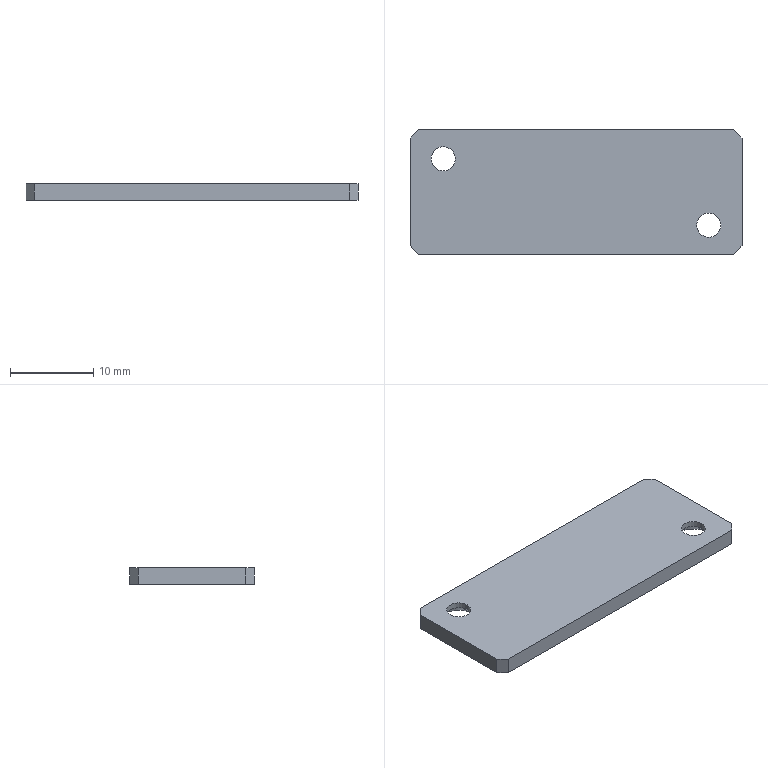Part | NX | features BREP 1 | 1 solid | 18 faces | box 40 x 15 x 2 mm | volume 1150 mm3 | plane 10 | cone 4 | cylinder 4 | commonest cylinder face diameters 2.9 x4
STEP:
#1=CARTESIAN_POINT('',(20.,6.5,1.));
#2=VERTEX_POINT('',#1);
#3=CARTESIAN_POINT('',(19.,7.5,1.));
#4=VERTEX_POINT('',#3);
#5=CARTESIAN_POINT('',(13.25,13.25,1.));
#6=DIRECTION('',(-0.7071,0.7071,0.));
#7=VECTOR('',#6,1000.);
#8=LINE('',#5,#7);
#9=EDGE_CURVE('',#2,#4,#8,.T.);
#10=ORIENTED_EDGE('',*,*,#9,.F.);
#11=CARTESIAN_POINT('',(20.,6.5,-1.));
#12=VERTEX_POINT('',#11);
#13=CARTESIAN_POINT('',(20.,6.5,1.));
#14=DIRECTION('',(0.,0.,1.));
#15=VECTOR('',#14,1000.);
#16=LINE('',#13,#15);
#17=EDGE_CURVE('',#12,#2,#16,.T.);
#18=ORIENTED_EDGE('',*,*,#17,.F.);
#19=CARTESIAN_POINT('',(19.,7.5,-1.));
#20=VERTEX_POINT('',#19);
#21=CARTESIAN_POINT('',(19.,7.5,-1.));
#22=DIRECTION('',(0.7071,-0.7071,0.));
#23=VECTOR('',#22,1000.);
#24=LINE('',#21,#23);
#25=EDGE_CURVE('',#20,#12,#24,.T.);
#26=ORIENTED_EDGE('',*,*,#25,.F.);
#27=CARTESIAN_POINT('',(19.,7.5,-1.));
#28=DIRECTION('',(0.,0.,-1.));
#29=VECTOR('',#28,1000.);
#30=LINE('',#27,#29);
#31=EDGE_CURVE('',#4,#20,#30,.T.);
#32=ORIENTED_EDGE('',*,*,#31,.F.);
#33=EDGE_LOOP('',(#10,#18,#26,#32));
#34=FACE_BOUND('',#33,.T.);
#35=CARTESIAN_POINT('',(19.,7.5,1.));
#36=DIRECTION('',(0.7071,0.7071,0.));
#37=DIRECTION('',(0.,0.,1.));
#38=AXIS2_PLACEMENT_3D('',#35,#36,#37);
#39=PLANE('',#38);
#40=ADVANCED_FACE('',(#34),#39,.T.);
#41=CARTESIAN_POINT('',(19.,-7.5,1.));
#42=VERTEX_POINT('',#41);
#43=CARTESIAN_POINT('',(20.,-6.5,1.));
#44=VERTEX_POINT('',#43);
#45=CARTESIAN_POINT('',(13.25,-13.25,1.));
#46=DIRECTION('',(0.7071,0.7071,0.));
#47=VECTOR('',#46,1000.);
#48=LINE('',#45,#47);
#49=EDGE_CURVE('',#42,#44,#48,.T.);
#50=ORIENTED_EDGE('',*,*,#49,.F.);
#51=CARTESIAN_POINT('',(19.,-7.5,-1.));
#52=VERTEX_POINT('',#51);
#53=CARTESIAN_POINT('',(19.,-7.5,1.));
#54=DIRECTION('',(0.,0.,1.));
#55=VECTOR('',#54,1000.);
#56=LINE('',#53,#55);
#57=EDGE_CURVE('',#52,#42,#56,.T.);
#58=ORIENTED_EDGE('',*,*,#57,.F.);
#59=CARTESIAN_POINT('',(20.,-6.5,-1.));
#60=VERTEX_POINT('',#59);
#61=CARTESIAN_POINT('',(20.,-6.5,-1.));
#62=DIRECTION('',(-0.7071,-0.7071,0.));
#63=VECTOR('',#62,1000.);
#64=LINE('',#61,#63);
#65=EDGE_CURVE('',#60,#52,#64,.T.);
#66=ORIENTED_EDGE('',*,*,#65,.F.);
#67=CARTESIAN_POINT('',(20.,-6.5,1.));
#68=DIRECTION('',(0.,0.,-1.));
#69=VECTOR('',#68,1000.);
#70=LINE('',#67,#69);
#71=EDGE_CURVE('',#44,#60,#70,.T.);
#72=ORIENTED_EDGE('',*,*,#71,.F.);
#73=EDGE_LOOP('',(#50,#58,#66,#72));
#74=FACE_BOUND('',#73,.T.);
#75=CARTESIAN_POINT('',(20.,-6.5,1.));
#76=DIRECTION('',(-0.7071,0.7071,0.));
#77=DIRECTION('',(0.,0.,-1.));
#78=AXIS2_PLACEMENT_3D('',#75,#76,#77);
#79=PLANE('',#78);
#80=ADVANCED_FACE('',(#74),#79,.F.);
#81=CARTESIAN_POINT('',(-19.,7.5,1.));
#82=VERTEX_POINT('',#81);
#83=CARTESIAN_POINT('',(-20.,6.5,1.));
#84=VERTEX_POINT('',#83);
#85=CARTESIAN_POINT('',(-13.25,13.25,1.));
#86=DIRECTION('',(-0.7071,-0.7071,0.));
#87=VECTOR('',#86,1000.);
#88=LINE('',#85,#87);
#89=EDGE_CURVE('',#82,#84,#88,.T.);
#90=ORIENTED_EDGE('',*,*,#89,.F.);
#91=CARTESIAN_POINT('',(-19.,7.5,-1.));
#92=VERTEX_POINT('',#91);
#93=CARTESIAN_POINT('',(-19.,7.5,1.));
#94=DIRECTION('',(0.,0.,1.));
#95=VECTOR('',#94,1000.);
#96=LINE('',#93,#95);
#97=EDGE_CURVE('',#92,#82,#96,.T.);
#98=ORIENTED_EDGE('',*,*,#97,.F.);
#99=CARTESIAN_POINT('',(-20.,6.5,-1.));
#100=VERTEX_POINT('',#99);
#101=CARTESIAN_POINT('',(-20.,6.5,-1.));
#102=DIRECTION('',(0.7071,0.7071,0.));
#103=VECTOR('',#102,1000.);
#104=LINE('',#101,#103);
#105=EDGE_CURVE('',#100,#92,#104,.T.);
#106=ORIENTED_EDGE('',*,*,#105,.F.);
#107=CARTESIAN_POINT('',(-20.,6.5,1.));
#108=DIRECTION('',(0.,0.,-1.));
#109=VECTOR('',#108,1000.);
#110=LINE('',#107,#109);
#111=EDGE_CURVE('',#84,#100,#110,.T.);
#112=ORIENTED_EDGE('',*,*,#111,.F.);
#113=EDGE_LOOP('',(#90,#98,#106,#112));
#114=FACE_BOUND('',#113,.T.);
#115=CARTESIAN_POINT('',(-20.,6.5,1.));
#116=DIRECTION('',(0.7071,-0.7071,0.));
#117=DIRECTION('',(0.,0.,-1.));
#118=AXIS2_PLACEMENT_3D('',#115,#116,#117);
#119=PLANE('',#118);
#120=ADVANCED_FACE('',(#114),#119,.F.);
#121=CARTESIAN_POINT('',(-20.,-6.5,1.));
#122=VERTEX_POINT('',#121);
#123=CARTESIAN_POINT('',(-19.,-7.5,1.));
#124=VERTEX_POINT('',#123);
#125=CARTESIAN_POINT('',(-13.25,-13.25,1.));
#126=DIRECTION('',(0.7071,-0.7071,0.));
#127=VECTOR('',#126,1000.);
#128=LINE('',#125,#127);
#129=EDGE_CURVE('',#122,#124,#128,.T.);
#130=ORIENTED_EDGE('',*,*,#129,.F.);
#131=CARTESIAN_POINT('',(-20.,-6.5,-1.));
#132=VERTEX_POINT('',#131);
#133=CARTESIAN_POINT('',(-20.,-6.5,1.));
#134=DIRECTION('',(0.,0.,1.));
#135=VECTOR('',#134,1000.);
#136=LINE('',#133,#135);
#137=EDGE_CURVE('',#132,#122,#136,.T.);
#138=ORIENTED_EDGE('',*,*,#137,.F.);
#139=CARTESIAN_POINT('',(-19.,-7.5,-1.));
#140=VERTEX_POINT('',#139);
#141=CARTESIAN_POINT('',(-19.,-7.5,-1.));
#142=DIRECTION('',(-0.7071,0.7071,0.));
#143=VECTOR('',#142,1000.);
#144=LINE('',#141,#143);
#145=EDGE_CURVE('',#140,#132,#144,.T.);
#146=ORIENTED_EDGE('',*,*,#145,.F.);
#147=CARTESIAN_POINT('',(-19.,-7.5,-1.));
#148=DIRECTION('',(0.,0.,-1.));
#149=VECTOR('',#148,1000.);
#150=LINE('',#147,#149);
#151=EDGE_CURVE('',#124,#140,#150,.T.);
#152=ORIENTED_EDGE('',*,*,#151,.F.);
#153=EDGE_LOOP('',(#130,#138,#146,#152));
#154=FACE_BOUND('',#153,.T.);
#155=CARTESIAN_POINT('',(-19.,-7.5,1.));
#156=DIRECTION('',(-0.7071,-0.7071,0.));
#157=DIRECTION('',(0.,0.,1.));
#158=AXIS2_PLACEMENT_3D('',#155,#156,#157);
#159=PLANE('',#158);
#160=ADVANCED_FACE('',(#154),#159,.T.);
#161=CARTESIAN_POINT('',(-14.55,4.,0.3));
#162=VERTEX_POINT('',#161);
#163=CARTESIAN_POINT('',(-13.25,4.,-1.));
#164=VERTEX_POINT('',#163);
#165=CARTESIAN_POINT('',(-13.25,4.,-1.));
#166=DIRECTION('',(0.7071,0.,-0.7071));
#167=VECTOR('',#166,1000.);
#168=LINE('',#165,#167);
#169=EDGE_CURVE('',#162,#164,#168,.T.);
#170=ORIENTED_EDGE('',*,*,#169,.F.);
#171=CARTESIAN_POINT('',(-17.45,4.,0.3));
#172=VERTEX_POINT('',#171);
#173=CARTESIAN_POINT('',(-16.,4.,0.3));
#174=DIRECTION('',(0.,0.,-1.));
#175=DIRECTION('',(-1.,0.,0.));
#176=AXIS2_PLACEMENT_3D('',#173,#174,#175);
#177=CIRCLE('',#176,1.45);
#178=EDGE_CURVE('',#172,#162,#177,.T.);
#179=ORIENTED_EDGE('',*,*,#178,.F.);
#180=CARTESIAN_POINT('',(-18.75,4.,-1.));
#181=VERTEX_POINT('',#180);
#182=CARTESIAN_POINT('',(-18.75,4.,-1.));
#183=DIRECTION('',(-0.7071,0.,-0.7071));
#184=VECTOR('',#183,1000.);
#185=LINE('',#182,#184);
#186=EDGE_CURVE('',#172,#181,#185,.T.);
#187=ORIENTED_EDGE('',*,*,#186,.T.);
#188=CARTESIAN_POINT('',(-16.,4.,-1.));
#189=DIRECTION('',(0.,0.,-1.));
#190=DIRECTION('',(-1.,0.,0.));
#191=AXIS2_PLACEMENT_3D('',#188,#189,#190);
#192=CIRCLE('',#191,2.75);
#193=EDGE_CURVE('',#181,#164,#192,.T.);
#194=ORIENTED_EDGE('',*,*,#193,.T.);
#195=EDGE_LOOP('',(#170,#179,#187,#194));
#196=FACE_BOUND('',#195,.T.);
#197=CARTESIAN_POINT('',(-16.,4.,-1.));
#198=DIRECTION('',(0.,0.,-1.));
#199=DIRECTION('',(-1.,0.,0.));
#200=AXIS2_PLACEMENT_3D('',#197,#198,#199);
#201=CONICAL_SURFACE('',#200,2.75,0.7854);
#202=ADVANCED_FACE('',(#196),#201,.F.);
#203=CARTESIAN_POINT('',(-14.55,4.,1.));
#204=VERTEX_POINT('',#203);
#205=CARTESIAN_POINT('',(-14.55,4.,-1.));
#206=DIRECTION('',(0.,0.,-1.));
#207=VECTOR('',#206,1000.);
#208=LINE('',#205,#207);
#209=EDGE_CURVE('',#204,#162,#208,.T.);
#210=ORIENTED_EDGE('',*,*,#209,.F.);
#211=CARTESIAN_POINT('',(-17.45,4.,1.));
#212=VERTEX_POINT('',#211);
#213=CARTESIAN_POINT('',(-16.,4.,1.));
#214=DIRECTION('',(0.,0.,-1.));
#215=DIRECTION('',(-1.,0.,0.));
#216=AXIS2_PLACEMENT_3D('',#213,#214,#215);
#217=CIRCLE('',#216,1.45);
#218=EDGE_CURVE('',#212,#204,#217,.T.);
#219=ORIENTED_EDGE('',*,*,#218,.F.);
#220=CARTESIAN_POINT('',(-17.45,4.,-1.));
#221=DIRECTION('',(0.,0.,-1.));
#222=VECTOR('',#221,1000.);
#223=LINE('',#220,#222);
#224=EDGE_CURVE('',#212,#172,#223,.T.);
#225=ORIENTED_EDGE('',*,*,#224,.T.);
#226=ORIENTED_EDGE('',*,*,#178,.T.);
#227=EDGE_LOOP('',(#210,#219,#225,#226));
#228=FACE_BOUND('',#227,.T.);
#229=CARTESIAN_POINT('',(-16.,4.,-1.));
#230=DIRECTION('',(0.,0.,-1.));
#231=DIRECTION('',(-1.,0.,0.));
#232=AXIS2_PLACEMENT_3D('',#229,#230,#231);
#233=CYLINDRICAL_SURFACE('',#232,1.45);
#234=ADVANCED_FACE('',(#228),#233,.F.);
#235=CARTESIAN_POINT('',(17.45,-4.,0.3));
#236=VERTEX_POINT('',#235);
#237=CARTESIAN_POINT('',(18.75,-4.,-1.));
#238=VERTEX_POINT('',#237);
#239=CARTESIAN_POINT('',(18.75,-4.,-1.));
#240=DIRECTION('',(0.7071,0.,-0.7071));
#241=VECTOR('',#240,1000.);
#242=LINE('',#239,#241);
#243=EDGE_CURVE('',#236,#238,#242,.T.);
#244=ORIENTED_EDGE('',*,*,#243,.F.);
#245=CARTESIAN_POINT('',(14.55,-4.,0.3));
#246=VERTEX_POINT('',#245);
#247=CARTESIAN_POINT('',(16.,-4.,0.3));
#248=DIRECTION('',(0.,0.,-1.));
#249=DIRECTION('',(-1.,0.,0.));
#250=AXIS2_PLACEMENT_3D('',#247,#248,#249);
#251=CIRCLE('',#250,1.45);
#252=EDGE_CURVE('',#246,#236,#251,.T.);
#253=ORIENTED_EDGE('',*,*,#252,.F.);
#254=CARTESIAN_POINT('',(13.25,-4.,-1.));
#255=VERTEX_POINT('',#254);
#256=CARTESIAN_POINT('',(13.25,-4.,-1.));
#257=DIRECTION('',(-0.7071,0.,-0.7071));
#258=VECTOR('',#257,1000.);
#259=LINE('',#256,#258);
#260=EDGE_CURVE('',#246,#255,#259,.T.);
#261=ORIENTED_EDGE('',*,*,#260,.T.);
#262=CARTESIAN_POINT('',(16.,-4.,-1.));
#263=DIRECTION('',(0.,0.,-1.));
#264=DIRECTION('',(-1.,0.,0.));
#265=AXIS2_PLACEMENT_3D('',#262,#263,#264);
#266=CIRCLE('',#265,2.75);
#267=EDGE_CURVE('',#255,#238,#266,.T.);
#268=ORIENTED_EDGE('',*,*,#267,.T.);
#269=EDGE_LOOP('',(#244,#253,#261,#268));
#270=FACE_BOUND('',#269,.T.);
#271=CARTESIAN_POINT('',(16.,-4.,-1.));
#272=DIRECTION('',(0.,0.,-1.));
#273=DIRECTION('',(-1.,0.,0.));
#274=AXIS2_PLACEMENT_3D('',#271,#272,#273);
#275=CONICAL_SURFACE('',#274,2.75,0.7854);
#276=ADVANCED_FACE('',(#270),#275,.F.);
#277=CARTESIAN_POINT('',(17.45,-4.,1.));
#278=VERTEX_POINT('',#277);
#279=CARTESIAN_POINT('',(17.45,-4.,-1.));
#280=DIRECTION('',(0.,0.,-1.));
#281=VECTOR('',#280,1000.);
#282=LINE('',#279,#281);
#283=EDGE_CURVE('',#278,#236,#282,.T.);
#284=ORIENTED_EDGE('',*,*,#283,.F.);
#285=CARTESIAN_POINT('',(14.55,-4.,1.));
#286=VERTEX_POINT('',#285);
#287=CARTESIAN_POINT('',(16.,-4.,1.));
#288=DIRECTION('',(0.,0.,-1.));
#289=DIRECTION('',(-1.,0.,0.));
#290=AXIS2_PLACEMENT_3D('',#287,#288,#289);
#291=CIRCLE('',#290,1.45);
#292=EDGE_CURVE('',#286,#278,#291,.T.);
#293=ORIENTED_EDGE('',*,*,#292,.F.);
#294=CARTESIAN_POINT('',(14.55,-4.,-1.));
#295=DIRECTION('',(0.,0.,-1.));
#296=VECTOR('',#295,1000.);
#297=LINE('',#294,#296);
#298=EDGE_CURVE('',#286,#246,#297,.T.);
#299=ORIENTED_EDGE('',*,*,#298,.T.);
#300=ORIENTED_EDGE('',*,*,#252,.T.);
#301=EDGE_LOOP('',(#284,#293,#299,#300));
#302=FACE_BOUND('',#301,.T.);
#303=CARTESIAN_POINT('',(16.,-4.,-1.));
#304=DIRECTION('',(0.,0.,-1.));
#305=DIRECTION('',(-1.,0.,0.));
#306=AXIS2_PLACEMENT_3D('',#303,#304,#305);
#307=CYLINDRICAL_SURFACE('',#306,1.45);
#308=ADVANCED_FACE('',(#302),#307,.F.);
#309=CARTESIAN_POINT('',(0.,-7.5,-1.));
#310=DIRECTION('',(1.,0.,0.));
#311=VECTOR('',#310,1000.);
#312=LINE('',#309,#311);
#313=EDGE_CURVE('',#140,#52,#312,.T.);
#314=ORIENTED_EDGE('',*,*,#313,.F.);
#315=ORIENTED_EDGE('',*,*,#145,.T.);
#316=CARTESIAN_POINT('',(-20.,0.,-1.));
#317=DIRECTION('',(0.,1.,0.));
#318=VECTOR('',#317,1000.);
#319=LINE('',#316,#318);
#320=EDGE_CURVE('',#132,#100,#319,.T.);
#321=ORIENTED_EDGE('',*,*,#320,.T.);
#322=ORIENTED_EDGE('',*,*,#105,.T.);
#323=CARTESIAN_POINT('',(0.,7.5,-1.));
#324=DIRECTION('',(1.,0.,0.));
#325=VECTOR('',#324,1000.);
#326=LINE('',#323,#325);
#327=EDGE_CURVE('',#92,#20,#326,.T.);
#328=ORIENTED_EDGE('',*,*,#327,.T.);
#329=ORIENTED_EDGE('',*,*,#25,.T.);
#330=CARTESIAN_POINT('',(20.,0.,-1.));
#331=DIRECTION('',(0.,1.,0.));
#332=VECTOR('',#331,1000.);
#333=LINE('',#330,#332);
#334=EDGE_CURVE('',#60,#12,#333,.T.);
#335=ORIENTED_EDGE('',*,*,#334,.F.);
#336=ORIENTED_EDGE('',*,*,#65,.T.);
#337=EDGE_LOOP('',(#314,#315,#321,#322,#328,#329,#335,#336));
#338=FACE_BOUND('',#337,.T.);
#339=ORIENTED_EDGE('',*,*,#267,.F.);
#340=CARTESIAN_POINT('',(16.,-4.,-1.));
#341=DIRECTION('',(0.,0.,-1.));
#342=DIRECTION('',(-1.,0.,0.));
#343=AXIS2_PLACEMENT_3D('',#340,#341,#342);
#344=CIRCLE('',#343,2.75);
#345=EDGE_CURVE('',#238,#255,#344,.T.);
#346=ORIENTED_EDGE('',*,*,#345,.F.);
#347=EDGE_LOOP('',(#339,#346));
#348=FACE_BOUND('',#347,.T.);
#349=ORIENTED_EDGE('',*,*,#193,.F.);
#350=CARTESIAN_POINT('',(-16.,4.,-1.));
#351=DIRECTION('',(0.,0.,-1.));
#352=DIRECTION('',(-1.,0.,0.));
#353=AXIS2_PLACEMENT_3D('',#350,#351,#352);
#354=CIRCLE('',#353,2.75);
#355=EDGE_CURVE('',#164,#181,#354,.T.);
#356=ORIENTED_EDGE('',*,*,#355,.F.);
#357=EDGE_LOOP('',(#349,#356));
#358=FACE_BOUND('',#357,.T.);
#359=CARTESIAN_POINT('',(0.,0.,-1.));
#360=DIRECTION('',(0.,0.,1.));
#361=DIRECTION('',(1.,0.,0.));
#362=AXIS2_PLACEMENT_3D('',#359,#360,#361);
#363=PLANE('',#362);
#364=ADVANCED_FACE('',(#338,#348,#358),#363,.F.);
#365=CARTESIAN_POINT('',(-20.,0.,1.));
#366=DIRECTION('',(0.,1.,0.));
#367=VECTOR('',#366,1000.);
#368=LINE('',#365,#367);
#369=EDGE_CURVE('',#122,#84,#368,.T.);
#370=ORIENTED_EDGE('',*,*,#369,.F.);
#371=ORIENTED_EDGE('',*,*,#129,.T.);
#372=CARTESIAN_POINT('',(0.,-7.5,1.));
#373=DIRECTION('',(1.,0.,0.));
#374=VECTOR('',#373,1000.);
#375=LINE('',#372,#374);
#376=EDGE_CURVE('',#124,#42,#375,.T.);
#377=ORIENTED_EDGE('',*,*,#376,.T.);
#378=ORIENTED_EDGE('',*,*,#49,.T.);
#379=CARTESIAN_POINT('',(20.,0.,1.));
#380=DIRECTION('',(0.,1.,0.));
#381=VECTOR('',#380,1000.);
#382=LINE('',#379,#381);
#383=EDGE_CURVE('',#44,#2,#382,.T.);
#384=ORIENTED_EDGE('',*,*,#383,.T.);
#385=ORIENTED_EDGE('',*,*,#9,.T.);
#386=CARTESIAN_POINT('',(0.,7.5,1.));
#387=DIRECTION('',(1.,0.,0.));
#388=VECTOR('',#387,1000.);
#389=LINE('',#386,#388);
#390=EDGE_CURVE('',#82,#4,#389,.T.);
#391=ORIENTED_EDGE('',*,*,#390,.F.);
#392=ORIENTED_EDGE('',*,*,#89,.T.);
#393=EDGE_LOOP('',(#370,#371,#377,#378,#384,#385,#391,#392));
#394=FACE_BOUND('',#393,.T.);
#395=ORIENTED_EDGE('',*,*,#292,.T.);
#396=CARTESIAN_POINT('',(16.,-4.,1.));
#397=DIRECTION('',(0.,0.,-1.));
#398=DIRECTION('',(-1.,0.,0.));
#399=AXIS2_PLACEMENT_3D('',#396,#397,#398);
#400=CIRCLE('',#399,1.45);
#401=EDGE_CURVE('',#278,#286,#400,.T.);
#402=ORIENTED_EDGE('',*,*,#401,.T.);
#403=EDGE_LOOP('',(#395,#402));
#404=FACE_BOUND('',#403,.T.);
#405=ORIENTED_EDGE('',*,*,#218,.T.);
#406=CARTESIAN_POINT('',(-16.,4.,1.));
#407=DIRECTION('',(0.,0.,-1.));
#408=DIRECTION('',(-1.,0.,0.));
#409=AXIS2_PLACEMENT_3D('',#406,#407,#408);
#410=CIRCLE('',#409,1.45);
#411=EDGE_CURVE('',#204,#212,#410,.T.);
#412=ORIENTED_EDGE('',*,*,#411,.T.);
#413=EDGE_LOOP('',(#405,#412));
#414=FACE_BOUND('',#413,.T.);
#415=CARTESIAN_POINT('',(0.,0.,1.));
#416=DIRECTION('',(0.,0.,1.));
#417=DIRECTION('',(1.,0.,0.));
#418=AXIS2_PLACEMENT_3D('',#415,#416,#417);
#419=PLANE('',#418);
#420=ADVANCED_FACE('',(#394,#404,#414),#419,.T.);
#421=ORIENTED_EDGE('',*,*,#320,.F.);
#422=ORIENTED_EDGE('',*,*,#137,.T.);
#423=ORIENTED_EDGE('',*,*,#369,.T.);
#424=ORIENTED_EDGE('',*,*,#111,.T.);
#425=EDGE_LOOP('',(#421,#422,#423,#424));
#426=FACE_BOUND('',#425,.T.);
#427=CARTESIAN_POINT('',(-20.,0.,1.));
#428=DIRECTION('',(-1.,0.,0.));
#429=DIRECTION('',(0.,0.,1.));
#430=AXIS2_PLACEMENT_3D('',#427,#428,#429);
#431=PLANE('',#430);
#432=ADVANCED_FACE('',(#426),#431,.T.);
#433=ORIENTED_EDGE('',*,*,#327,.F.);
#434=ORIENTED_EDGE('',*,*,#97,.T.);
#435=ORIENTED_EDGE('',*,*,#390,.T.);
#436=ORIENTED_EDGE('',*,*,#31,.T.);
#437=EDGE_LOOP('',(#433,#434,#435,#436));
#438=FACE_BOUND('',#437,.T.);
#439=CARTESIAN_POINT('',(0.,7.5,1.));
#440=DIRECTION('',(0.,1.,0.));
#441=DIRECTION('',(0.,0.,1.));
#442=AXIS2_PLACEMENT_3D('',#439,#440,#441);
#443=PLANE('',#442);
#444=ADVANCED_FACE('',(#438),#443,.T.);
#445=ORIENTED_EDGE('',*,*,#383,.F.);
#446=ORIENTED_EDGE('',*,*,#71,.T.);
#447=ORIENTED_EDGE('',*,*,#334,.T.);
#448=ORIENTED_EDGE('',*,*,#17,.T.);
#449=EDGE_LOOP('',(#445,#446,#447,#448));
#450=FACE_BOUND('',#449,.T.);
#451=CARTESIAN_POINT('',(20.,0.,1.));
#452=DIRECTION('',(-1.,0.,0.));
#453=DIRECTION('',(0.,0.,1.));
#454=AXIS2_PLACEMENT_3D('',#451,#452,#453);
#455=PLANE('',#454);
#456=ADVANCED_FACE('',(#450),#455,.F.);
#457=ORIENTED_EDGE('',*,*,#376,.F.);
#458=ORIENTED_EDGE('',*,*,#151,.T.);
#459=ORIENTED_EDGE('',*,*,#313,.T.);
#460=ORIENTED_EDGE('',*,*,#57,.T.);
#461=EDGE_LOOP('',(#457,#458,#459,#460));
#462=FACE_BOUND('',#461,.T.);
#463=CARTESIAN_POINT('',(0.,-7.5,1.));
#464=DIRECTION('',(0.,1.,0.));
#465=DIRECTION('',(0.,0.,1.));
#466=AXIS2_PLACEMENT_3D('',#463,#464,#465);
#467=PLANE('',#466);
#468=ADVANCED_FACE('',(#462),#467,.F.);
#469=ORIENTED_EDGE('',*,*,#401,.F.);
#470=ORIENTED_EDGE('',*,*,#283,.T.);
#471=CARTESIAN_POINT('',(16.,-4.,0.3));
#472=DIRECTION('',(0.,0.,-1.));
#473=DIRECTION('',(-1.,0.,0.));
#474=AXIS2_PLACEMENT_3D('',#471,#472,#473);
#475=CIRCLE('',#474,1.45);
#476=EDGE_CURVE('',#236,#246,#475,.T.);
#477=ORIENTED_EDGE('',*,*,#476,.T.);
#478=ORIENTED_EDGE('',*,*,#298,.F.);
#479=EDGE_LOOP('',(#469,#470,#477,#478));
#480=FACE_BOUND('',#479,.T.);
#481=CARTESIAN_POINT('',(16.,-4.,-1.));
#482=DIRECTION('',(0.,0.,-1.));
#483=DIRECTION('',(-1.,0.,0.));
#484=AXIS2_PLACEMENT_3D('',#481,#482,#483);
#485=CYLINDRICAL_SURFACE('',#484,1.45);
#486=ADVANCED_FACE('',(#480),#485,.F.);
#487=ORIENTED_EDGE('',*,*,#476,.F.);
#488=ORIENTED_EDGE('',*,*,#243,.T.);
#489=ORIENTED_EDGE('',*,*,#345,.T.);
#490=ORIENTED_EDGE('',*,*,#260,.F.);
#491=EDGE_LOOP('',(#487,#488,#489,#490));
#492=FACE_BOUND('',#491,.T.);
#493=CARTESIAN_POINT('',(16.,-4.,-1.));
#494=DIRECTION('',(0.,0.,-1.));
#495=DIRECTION('',(-1.,0.,0.));
#496=AXIS2_PLACEMENT_3D('',#493,#494,#495);
#497=CONICAL_SURFACE('',#496,2.75,0.7854);
#498=ADVANCED_FACE('',(#492),#497,.F.);
#499=ORIENTED_EDGE('',*,*,#411,.F.);
#500=ORIENTED_EDGE('',*,*,#209,.T.);
#501=CARTESIAN_POINT('',(-16.,4.,0.3));
#502=DIRECTION('',(0.,0.,-1.));
#503=DIRECTION('',(-1.,0.,0.));
#504=AXIS2_PLACEMENT_3D('',#501,#502,#503);
#505=CIRCLE('',#504,1.45);
#506=EDGE_CURVE('',#162,#172,#505,.T.);
#507=ORIENTED_EDGE('',*,*,#506,.T.);
#508=ORIENTED_EDGE('',*,*,#224,.F.);
#509=EDGE_LOOP('',(#499,#500,#507,#508));
#510=FACE_BOUND('',#509,.T.);
#511=CARTESIAN_POINT('',(-16.,4.,-1.));
#512=DIRECTION('',(0.,0.,-1.));
#513=DIRECTION('',(-1.,0.,0.));
#514=AXIS2_PLACEMENT_3D('',#511,#512,#513);
#515=CYLINDRICAL_SURFACE('',#514,1.45);
#516=ADVANCED_FACE('',(#510),#515,.F.);
#517=ORIENTED_EDGE('',*,*,#506,.F.);
#518=ORIENTED_EDGE('',*,*,#169,.T.);
#519=ORIENTED_EDGE('',*,*,#355,.T.);
#520=ORIENTED_EDGE('',*,*,#186,.F.);
#521=EDGE_LOOP('',(#517,#518,#519,#520));
#522=FACE_BOUND('',#521,.T.);
#523=CARTESIAN_POINT('',(-16.,4.,-1.));
#524=DIRECTION('',(0.,0.,-1.));
#525=DIRECTION('',(-1.,0.,0.));
#526=AXIS2_PLACEMENT_3D('',#523,#524,#525);
#527=CONICAL_SURFACE('',#526,2.75,0.7854);
#528=ADVANCED_FACE('',(#522),#527,.F.);
#529=CLOSED_SHELL('',(#40,#80,#120,#160,#202,#234,#276,#308,#364,#420,#432,#444,#456,#468,#486,#498,#516,#528));
#530=MANIFOLD_SOLID_BREP('',#529);
#531=(LENGTH_UNIT()NAMED_UNIT(*)SI_UNIT(.MILLI.,.METRE.));
#532=UNCERTAINTY_MEASURE_WITH_UNIT(LENGTH_MEASURE(0.00001),#531,'','');
#533=(NAMED_UNIT(*)PLANE_ANGLE_UNIT()SI_UNIT($,.RADIAN.));
#534=(NAMED_UNIT(*)SI_UNIT($,.STERADIAN.)SOLID_ANGLE_UNIT());
#535=(GEOMETRIC_REPRESENTATION_CONTEXT(3)GLOBAL_UNCERTAINTY_ASSIGNED_CONTEXT((#532))GLOBAL_UNIT_ASSIGNED_CONTEXT((#531,#533,#534))REPRESENTATION_CONTEXT('',''));
#536=ADVANCED_BREP_SHAPE_REPRESENTATION('',(#530),#535);